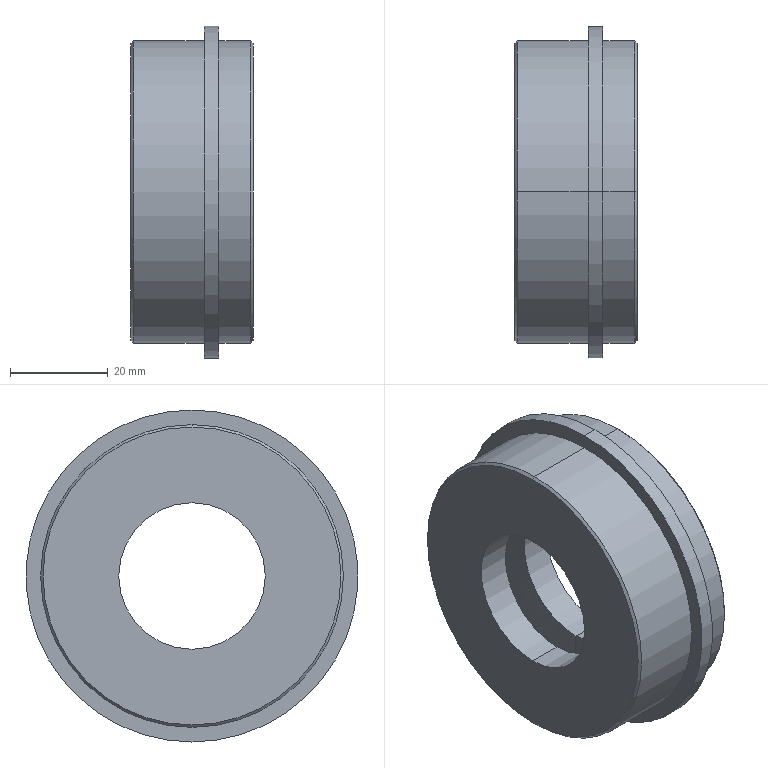Part | SolidWorks | features MBimport 1 | 1 solid | 29 faces | box 25 x 68 x 68 mm | volume 46745 mm3 | cylinder 14 | cone 8 | plane 5 | torus 2 | commonest cylinder face diameters 30 x4 62 x4 46 x2 52 x2 68 x2
STEP:
#1=CARTESIAN_POINT('',(25.,0.,-30.5));
#2=VERTEX_POINT('',#1);
#3=CARTESIAN_POINT('',(25.,0.,30.5));
#4=VERTEX_POINT('',#3);
#5=CARTESIAN_POINT('',(25.,0.,0.));
#6=DIRECTION('',(1.,0.,0.));
#7=DIRECTION('',(0.,0.,1.));
#8=AXIS2_PLACEMENT_3D('',#5,#6,#7);
#9=CIRCLE('',#8,30.5);
#10=EDGE_CURVE('',#2,#4,#9,.T.);
#11=ORIENTED_EDGE('',*,*,#10,.F.);
#12=CARTESIAN_POINT('',(24.5,0.,-31.));
#13=VERTEX_POINT('',#12);
#14=CARTESIAN_POINT('',(24.5,0.,-31.));
#15=DIRECTION('',(-0.7071,0.,-0.7071));
#16=VECTOR('',#15,1000.);
#17=LINE('',#14,#16);
#18=EDGE_CURVE('',#2,#13,#17,.T.);
#19=ORIENTED_EDGE('',*,*,#18,.T.);
#20=CARTESIAN_POINT('',(24.5,0.,31.));
#21=VERTEX_POINT('',#20);
#22=CARTESIAN_POINT('',(24.5,0.,0.));
#23=DIRECTION('',(-1.,0.,0.));
#24=DIRECTION('',(0.,0.,1.));
#25=AXIS2_PLACEMENT_3D('',#22,#23,#24);
#26=CIRCLE('',#25,31.);
#27=EDGE_CURVE('',#21,#13,#26,.T.);
#28=ORIENTED_EDGE('',*,*,#27,.F.);
#29=CARTESIAN_POINT('',(24.5,0.,31.));
#30=DIRECTION('',(-0.7071,0.,0.7071));
#31=VECTOR('',#30,1000.);
#32=LINE('',#29,#31);
#33=EDGE_CURVE('',#4,#21,#32,.T.);
#34=ORIENTED_EDGE('',*,*,#33,.F.);
#35=EDGE_LOOP('',(#11,#19,#28,#34));
#36=FACE_OUTER_BOUND('',#35,.T.);
#37=CARTESIAN_POINT('',(24.5,0.,0.));
#38=DIRECTION('',(-1.,0.,0.));
#39=DIRECTION('',(0.,0.,1.));
#40=AXIS2_PLACEMENT_3D('',#37,#38,#39);
#41=CONICAL_SURFACE('',#40,31.,0.7854);
#42=ADVANCED_FACE('',(#36),#41,.T.);
#43=CARTESIAN_POINT('',(0.,0.,30.5));
#44=VERTEX_POINT('',#43);
#45=CARTESIAN_POINT('',(0.,0.,-30.5));
#46=VERTEX_POINT('',#45);
#47=CARTESIAN_POINT('',(0.,0.,0.));
#48=DIRECTION('',(-1.,0.,0.));
#49=DIRECTION('',(0.,0.,-1.));
#50=AXIS2_PLACEMENT_3D('',#47,#48,#49);
#51=CIRCLE('',#50,30.5);
#52=EDGE_CURVE('',#44,#46,#51,.T.);
#53=ORIENTED_EDGE('',*,*,#52,.F.);
#54=CARTESIAN_POINT('',(0.5,0.,31.));
#55=VERTEX_POINT('',#54);
#56=CARTESIAN_POINT('',(0.,0.,30.5));
#57=DIRECTION('',(0.7071,0.,0.7071));
#58=VECTOR('',#57,1000.);
#59=LINE('',#56,#58);
#60=EDGE_CURVE('',#44,#55,#59,.T.);
#61=ORIENTED_EDGE('',*,*,#60,.T.);
#62=CARTESIAN_POINT('',(0.5,0.,-31.));
#63=VERTEX_POINT('',#62);
#64=CARTESIAN_POINT('',(0.5,0.,0.));
#65=DIRECTION('',(1.,0.,0.));
#66=DIRECTION('',(0.,0.,-1.));
#67=AXIS2_PLACEMENT_3D('',#64,#65,#66);
#68=CIRCLE('',#67,31.);
#69=EDGE_CURVE('',#63,#55,#68,.T.);
#70=ORIENTED_EDGE('',*,*,#69,.F.);
#71=CARTESIAN_POINT('',(0.,0.,-30.5));
#72=DIRECTION('',(0.7071,0.,-0.7071));
#73=VECTOR('',#72,1000.);
#74=LINE('',#71,#73);
#75=EDGE_CURVE('',#46,#63,#74,.T.);
#76=ORIENTED_EDGE('',*,*,#75,.F.);
#77=EDGE_LOOP('',(#53,#61,#70,#76));
#78=FACE_OUTER_BOUND('',#77,.T.);
#79=CARTESIAN_POINT('',(0.,0.,0.));
#80=DIRECTION('',(1.,0.,0.));
#81=DIRECTION('',(0.,0.,-1.));
#82=AXIS2_PLACEMENT_3D('',#79,#80,#81);
#83=CONICAL_SURFACE('',#82,30.5,0.7854);
#84=ADVANCED_FACE('',(#78),#83,.T.);
#85=CARTESIAN_POINT('',(21.,0.,-26.));
#86=VERTEX_POINT('',#85);
#87=CARTESIAN_POINT('',(21.,0.,26.));
#88=VERTEX_POINT('',#87);
#89=CARTESIAN_POINT('',(21.,0.,0.));
#90=DIRECTION('',(-1.,0.,0.));
#91=DIRECTION('',(0.,0.,1.));
#92=AXIS2_PLACEMENT_3D('',#89,#90,#91);
#93=CIRCLE('',#92,26.);
#94=EDGE_CURVE('',#86,#88,#93,.T.);
#95=ORIENTED_EDGE('',*,*,#94,.F.);
#96=CARTESIAN_POINT('',(19.,0.,-24.));
#97=VERTEX_POINT('',#96);
#98=CARTESIAN_POINT('',(21.,0.,-24.));
#99=DIRECTION('',(0.,1.,0.));
#100=DIRECTION('',(0.,0.,1.));
#101=AXIS2_PLACEMENT_3D('',#98,#99,#100);
#102=CIRCLE('',#101,2.);
#103=EDGE_CURVE('',#86,#97,#102,.T.);
#104=ORIENTED_EDGE('',*,*,#103,.T.);
#105=CARTESIAN_POINT('',(19.,0.,24.));
#106=VERTEX_POINT('',#105);
#107=CARTESIAN_POINT('',(19.,0.,0.));
#108=DIRECTION('',(1.,0.,0.));
#109=DIRECTION('',(0.,0.,1.));
#110=AXIS2_PLACEMENT_3D('',#107,#108,#109);
#111=CIRCLE('',#110,24.);
#112=EDGE_CURVE('',#106,#97,#111,.T.);
#113=ORIENTED_EDGE('',*,*,#112,.F.);
#114=CARTESIAN_POINT('',(21.,0.,24.));
#115=DIRECTION('',(0.,-1.,0.));
#116=DIRECTION('',(0.,0.,-1.));
#117=AXIS2_PLACEMENT_3D('',#114,#115,#116);
#118=CIRCLE('',#117,2.);
#119=EDGE_CURVE('',#88,#106,#118,.T.);
#120=ORIENTED_EDGE('',*,*,#119,.F.);
#121=EDGE_LOOP('',(#95,#104,#113,#120));
#122=FACE_OUTER_BOUND('',#121,.T.);
#123=CARTESIAN_POINT('',(21.,0.,0.));
#124=DIRECTION('',(-1.,0.,0.));
#125=DIRECTION('',(0.,0.,1.));
#126=AXIS2_PLACEMENT_3D('',#123,#124,#125);
#127=TOROIDAL_SURFACE('',#126,24.,2.);
#128=ADVANCED_FACE('',(#122),#127,.F.);
#129=CARTESIAN_POINT('',(15.,0.,31.));
#130=VERTEX_POINT('',#129);
#131=CARTESIAN_POINT('',(15.,0.,-31.));
#132=VERTEX_POINT('',#131);
#133=CARTESIAN_POINT('',(15.,0.,0.));
#134=DIRECTION('',(-1.,0.,0.));
#135=DIRECTION('',(0.,0.,1.));
#136=AXIS2_PLACEMENT_3D('',#133,#134,#135);
#137=CIRCLE('',#136,31.);
#138=EDGE_CURVE('',#130,#132,#137,.T.);
#139=ORIENTED_EDGE('',*,*,#138,.T.);
#140=CARTESIAN_POINT('',(0.,0.,-31.));
#141=DIRECTION('',(-1.,0.,0.));
#142=VECTOR('',#141,1000.);
#143=LINE('',#140,#142);
#144=EDGE_CURVE('',#132,#63,#143,.T.);
#145=ORIENTED_EDGE('',*,*,#144,.T.);
#146=ORIENTED_EDGE('',*,*,#69,.T.);
#147=CARTESIAN_POINT('',(0.,0.,31.));
#148=DIRECTION('',(-1.,0.,0.));
#149=VECTOR('',#148,1000.);
#150=LINE('',#147,#149);
#151=EDGE_CURVE('',#130,#55,#150,.T.);
#152=ORIENTED_EDGE('',*,*,#151,.F.);
#153=EDGE_LOOP('',(#139,#145,#146,#152));
#154=FACE_OUTER_BOUND('',#153,.T.);
#155=CARTESIAN_POINT('',(0.,0.,0.));
#156=DIRECTION('',(-1.,0.,0.));
#157=DIRECTION('',(0.,0.,1.));
#158=AXIS2_PLACEMENT_3D('',#155,#156,#157);
#159=CYLINDRICAL_SURFACE('',#158,31.);
#160=ADVANCED_FACE('',(#154),#159,.T.);
#161=CARTESIAN_POINT('',(18.,0.,34.));
#162=VERTEX_POINT('',#161);
#163=CARTESIAN_POINT('',(18.,0.,-34.));
#164=VERTEX_POINT('',#163);
#165=CARTESIAN_POINT('',(18.,0.,0.));
#166=DIRECTION('',(-1.,0.,0.));
#167=DIRECTION('',(0.,0.,1.));
#168=AXIS2_PLACEMENT_3D('',#165,#166,#167);
#169=CIRCLE('',#168,34.);
#170=EDGE_CURVE('',#162,#164,#169,.T.);
#171=ORIENTED_EDGE('',*,*,#170,.T.);
#172=CARTESIAN_POINT('',(15.,0.,-34.));
#173=VERTEX_POINT('',#172);
#174=CARTESIAN_POINT('',(0.,0.,-34.));
#175=DIRECTION('',(-1.,0.,0.));
#176=VECTOR('',#175,1000.);
#177=LINE('',#174,#176);
#178=EDGE_CURVE('',#164,#173,#177,.T.);
#179=ORIENTED_EDGE('',*,*,#178,.T.);
#180=CARTESIAN_POINT('',(15.,0.,34.));
#181=VERTEX_POINT('',#180);
#182=CARTESIAN_POINT('',(15.,0.,0.));
#183=DIRECTION('',(-1.,0.,0.));
#184=DIRECTION('',(0.,0.,1.));
#185=AXIS2_PLACEMENT_3D('',#182,#183,#184);
#186=CIRCLE('',#185,34.);
#187=EDGE_CURVE('',#181,#173,#186,.T.);
#188=ORIENTED_EDGE('',*,*,#187,.F.);
#189=CARTESIAN_POINT('',(0.,0.,34.));
#190=DIRECTION('',(-1.,0.,0.));
#191=VECTOR('',#190,1000.);
#192=LINE('',#189,#191);
#193=EDGE_CURVE('',#162,#181,#192,.T.);
#194=ORIENTED_EDGE('',*,*,#193,.F.);
#195=EDGE_LOOP('',(#171,#179,#188,#194));
#196=FACE_OUTER_BOUND('',#195,.T.);
#197=CARTESIAN_POINT('',(0.,0.,0.));
#198=DIRECTION('',(-1.,0.,0.));
#199=DIRECTION('',(0.,0.,1.));
#200=AXIS2_PLACEMENT_3D('',#197,#198,#199);
#201=CYLINDRICAL_SURFACE('',#200,34.);
#202=ADVANCED_FACE('',(#196),#201,.T.);
#203=ORIENTED_EDGE('',*,*,#27,.T.);
#204=CARTESIAN_POINT('',(18.,0.,-31.));
#205=VERTEX_POINT('',#204);
#206=CARTESIAN_POINT('',(0.,0.,-31.));
#207=DIRECTION('',(-1.,0.,0.));
#208=VECTOR('',#207,1000.);
#209=LINE('',#206,#208);
#210=EDGE_CURVE('',#13,#205,#209,.T.);
#211=ORIENTED_EDGE('',*,*,#210,.T.);
#212=CARTESIAN_POINT('',(18.,0.,31.));
#213=VERTEX_POINT('',#212);
#214=CARTESIAN_POINT('',(18.,0.,0.));
#215=DIRECTION('',(-1.,0.,0.));
#216=DIRECTION('',(0.,0.,1.));
#217=AXIS2_PLACEMENT_3D('',#214,#215,#216);
#218=CIRCLE('',#217,31.);
#219=EDGE_CURVE('',#213,#205,#218,.T.);
#220=ORIENTED_EDGE('',*,*,#219,.F.);
#221=CARTESIAN_POINT('',(0.,0.,31.));
#222=DIRECTION('',(-1.,0.,0.));
#223=VECTOR('',#222,1000.);
#224=LINE('',#221,#223);
#225=EDGE_CURVE('',#21,#213,#224,.T.);
#226=ORIENTED_EDGE('',*,*,#225,.F.);
#227=EDGE_LOOP('',(#203,#211,#220,#226));
#228=FACE_OUTER_BOUND('',#227,.T.);
#229=CARTESIAN_POINT('',(0.,0.,0.));
#230=DIRECTION('',(-1.,0.,0.));
#231=DIRECTION('',(0.,0.,1.));
#232=AXIS2_PLACEMENT_3D('',#229,#230,#231);
#233=CYLINDRICAL_SURFACE('',#232,31.);
#234=ADVANCED_FACE('',(#228),#233,.T.);
#235=CARTESIAN_POINT('',(25.,0.,-26.));
#236=VERTEX_POINT('',#235);
#237=CARTESIAN_POINT('',(25.,0.,26.));
#238=VERTEX_POINT('',#237);
#239=CARTESIAN_POINT('',(25.,0.,0.));
#240=DIRECTION('',(-1.,0.,0.));
#241=DIRECTION('',(0.,0.,1.));
#242=AXIS2_PLACEMENT_3D('',#239,#240,#241);
#243=CIRCLE('',#242,26.);
#244=EDGE_CURVE('',#236,#238,#243,.T.);
#245=ORIENTED_EDGE('',*,*,#244,.F.);
#246=CARTESIAN_POINT('',(0.,0.,-26.));
#247=DIRECTION('',(-1.,0.,0.));
#248=VECTOR('',#247,1000.);
#249=LINE('',#246,#248);
#250=EDGE_CURVE('',#236,#86,#249,.T.);
#251=ORIENTED_EDGE('',*,*,#250,.T.);
#252=ORIENTED_EDGE('',*,*,#94,.T.);
#253=CARTESIAN_POINT('',(0.,0.,26.));
#254=DIRECTION('',(-1.,0.,0.));
#255=VECTOR('',#254,1000.);
#256=LINE('',#253,#255);
#257=EDGE_CURVE('',#238,#88,#256,.T.);
#258=ORIENTED_EDGE('',*,*,#257,.F.);
#259=EDGE_LOOP('',(#245,#251,#252,#258));
#260=FACE_OUTER_BOUND('',#259,.T.);
#261=CARTESIAN_POINT('',(0.,0.,0.));
#262=DIRECTION('',(-1.,0.,0.));
#263=DIRECTION('',(0.,0.,1.));
#264=AXIS2_PLACEMENT_3D('',#261,#262,#263);
#265=CYLINDRICAL_SURFACE('',#264,26.);
#266=ADVANCED_FACE('',(#260),#265,.F.);
#267=CARTESIAN_POINT('',(19.,0.,-15.));
#268=VERTEX_POINT('',#267);
#269=CARTESIAN_POINT('',(19.,0.,15.));
#270=VERTEX_POINT('',#269);
#271=CARTESIAN_POINT('',(19.,0.,0.));
#272=DIRECTION('',(-1.,0.,0.));
#273=DIRECTION('',(0.,0.,1.));
#274=AXIS2_PLACEMENT_3D('',#271,#272,#273);
#275=CIRCLE('',#274,15.);
#276=EDGE_CURVE('',#268,#270,#275,.T.);
#277=ORIENTED_EDGE('',*,*,#276,.F.);
#278=CARTESIAN_POINT('',(12.5,0.,-15.));
#279=VERTEX_POINT('',#278);
#280=CARTESIAN_POINT('',(0.,0.,-15.));
#281=DIRECTION('',(-1.,0.,0.));
#282=VECTOR('',#281,1000.);
#283=LINE('',#280,#282);
#284=EDGE_CURVE('',#268,#279,#283,.T.);
#285=ORIENTED_EDGE('',*,*,#284,.T.);
#286=CARTESIAN_POINT('',(12.5,0.,15.));
#287=VERTEX_POINT('',#286);
#288=CARTESIAN_POINT('',(12.5,0.,0.));
#289=DIRECTION('',(-1.,0.,0.));
#290=DIRECTION('',(0.,0.,1.));
#291=AXIS2_PLACEMENT_3D('',#288,#289,#290);
#292=CIRCLE('',#291,15.);
#293=EDGE_CURVE('',#279,#287,#292,.T.);
#294=ORIENTED_EDGE('',*,*,#293,.T.);
#295=CARTESIAN_POINT('',(0.,0.,15.));
#296=DIRECTION('',(-1.,0.,0.));
#297=VECTOR('',#296,1000.);
#298=LINE('',#295,#297);
#299=EDGE_CURVE('',#270,#287,#298,.T.);
#300=ORIENTED_EDGE('',*,*,#299,.F.);
#301=EDGE_LOOP('',(#277,#285,#294,#300));
#302=FACE_OUTER_BOUND('',#301,.T.);
#303=CARTESIAN_POINT('',(0.,0.,0.));
#304=DIRECTION('',(-1.,0.,0.));
#305=DIRECTION('',(0.,0.,1.));
#306=AXIS2_PLACEMENT_3D('',#303,#304,#305);
#307=CYLINDRICAL_SURFACE('',#306,15.);
#308=ADVANCED_FACE('',(#302),#307,.F.);
#309=ORIENTED_EDGE('',*,*,#293,.F.);
#310=CARTESIAN_POINT('',(11.75,0.,-23.));
#311=VERTEX_POINT('',#310);
#312=CARTESIAN_POINT('',(11.75,0.,-23.));
#313=DIRECTION('',(-0.09334,0.,-0.9956));
#314=VECTOR('',#313,1000.);
#315=LINE('',#312,#314);
#316=EDGE_CURVE('',#279,#311,#315,.T.);
#317=ORIENTED_EDGE('',*,*,#316,.T.);
#318=CARTESIAN_POINT('',(11.75,0.,23.));
#319=VERTEX_POINT('',#318);
#320=CARTESIAN_POINT('',(11.75,0.,0.));
#321=DIRECTION('',(-1.,0.,0.));
#322=DIRECTION('',(0.,0.,1.));
#323=AXIS2_PLACEMENT_3D('',#320,#321,#322);
#324=CIRCLE('',#323,23.);
#325=EDGE_CURVE('',#311,#319,#324,.T.);
#326=ORIENTED_EDGE('',*,*,#325,.T.);
#327=CARTESIAN_POINT('',(11.75,0.,23.));
#328=DIRECTION('',(-0.09334,0.,0.9956));
#329=VECTOR('',#328,1000.);
#330=LINE('',#327,#329);
#331=EDGE_CURVE('',#287,#319,#330,.T.);
#332=ORIENTED_EDGE('',*,*,#331,.F.);
#333=EDGE_LOOP('',(#309,#317,#326,#332));
#334=FACE_OUTER_BOUND('',#333,.T.);
#335=CARTESIAN_POINT('',(11.75,0.,0.));
#336=DIRECTION('',(-1.,0.,0.));
#337=DIRECTION('',(0.,0.,1.));
#338=AXIS2_PLACEMENT_3D('',#335,#336,#337);
#339=CONICAL_SURFACE('',#338,23.,1.477);
#340=ADVANCED_FACE('',(#334),#339,.F.);
#341=ORIENTED_EDGE('',*,*,#325,.F.);
#342=CARTESIAN_POINT('',(7.75,0.,-23.));
#343=VERTEX_POINT('',#342);
#344=CARTESIAN_POINT('',(0.,0.,-23.));
#345=DIRECTION('',(-1.,0.,0.));
#346=VECTOR('',#345,1000.);
#347=LINE('',#344,#346);
#348=EDGE_CURVE('',#311,#343,#347,.T.);
#349=ORIENTED_EDGE('',*,*,#348,.T.);
#350=CARTESIAN_POINT('',(7.75,0.,23.));
#351=VERTEX_POINT('',#350);
#352=CARTESIAN_POINT('',(7.75,0.,0.));
#353=DIRECTION('',(-1.,0.,0.));
#354=DIRECTION('',(0.,0.,1.));
#355=AXIS2_PLACEMENT_3D('',#352,#353,#354);
#356=CIRCLE('',#355,23.);
#357=EDGE_CURVE('',#343,#351,#356,.T.);
#358=ORIENTED_EDGE('',*,*,#357,.T.);
#359=CARTESIAN_POINT('',(0.,0.,23.));
#360=DIRECTION('',(-1.,0.,0.));
#361=VECTOR('',#360,1000.);
#362=LINE('',#359,#361);
#363=EDGE_CURVE('',#319,#351,#362,.T.);
#364=ORIENTED_EDGE('',*,*,#363,.F.);
#365=EDGE_LOOP('',(#341,#349,#358,#364));
#366=FACE_OUTER_BOUND('',#365,.T.);
#367=CARTESIAN_POINT('',(0.,0.,0.));
#368=DIRECTION('',(-1.,0.,0.));
#369=DIRECTION('',(0.,0.,1.));
#370=AXIS2_PLACEMENT_3D('',#367,#368,#369);
#371=CYLINDRICAL_SURFACE('',#370,23.);
#372=ADVANCED_FACE('',(#366),#371,.F.);
#373=CARTESIAN_POINT('',(7.,0.,-15.));
#374=VERTEX_POINT('',#373);
#375=CARTESIAN_POINT('',(7.,0.,15.));
#376=VERTEX_POINT('',#375);
#377=CARTESIAN_POINT('',(7.,0.,0.));
#378=DIRECTION('',(-1.,0.,0.));
#379=DIRECTION('',(0.,0.,1.));
#380=AXIS2_PLACEMENT_3D('',#377,#378,#379);
#381=CIRCLE('',#380,15.);
#382=EDGE_CURVE('',#374,#376,#381,.T.);
#383=ORIENTED_EDGE('',*,*,#382,.T.);
#384=CARTESIAN_POINT('',(7.,0.,15.));
#385=DIRECTION('',(0.09334,0.,0.9956));
#386=VECTOR('',#385,1000.);
#387=LINE('',#384,#386);
#388=EDGE_CURVE('',#376,#351,#387,.T.);
#389=ORIENTED_EDGE('',*,*,#388,.T.);
#390=ORIENTED_EDGE('',*,*,#357,.F.);
#391=CARTESIAN_POINT('',(7.,0.,-15.));
#392=DIRECTION('',(0.09334,0.,-0.9956));
#393=VECTOR('',#392,1000.);
#394=LINE('',#391,#393);
#395=EDGE_CURVE('',#374,#343,#394,.T.);
#396=ORIENTED_EDGE('',*,*,#395,.F.);
#397=EDGE_LOOP('',(#383,#389,#390,#396));
#398=FACE_OUTER_BOUND('',#397,.T.);
#399=CARTESIAN_POINT('',(7.,0.,0.));
#400=DIRECTION('',(1.,0.,0.));
#401=DIRECTION('',(0.,0.,-1.));
#402=AXIS2_PLACEMENT_3D('',#399,#400,#401);
#403=CONICAL_SURFACE('',#402,15.,1.477);
#404=ADVANCED_FACE('',(#398),#403,.F.);
#405=ORIENTED_EDGE('',*,*,#382,.F.);
#406=CARTESIAN_POINT('',(0.,0.,-15.));
#407=VERTEX_POINT('',#406);
#408=CARTESIAN_POINT('',(0.,0.,-15.));
#409=DIRECTION('',(-1.,0.,0.));
#410=VECTOR('',#409,1000.);
#411=LINE('',#408,#410);
#412=EDGE_CURVE('',#374,#407,#411,.T.);
#413=ORIENTED_EDGE('',*,*,#412,.T.);
#414=CARTESIAN_POINT('',(0.,0.,15.));
#415=VERTEX_POINT('',#414);
#416=CARTESIAN_POINT('',(0.,0.,0.));
#417=DIRECTION('',(-1.,0.,0.));
#418=DIRECTION('',(0.,0.,1.));
#419=AXIS2_PLACEMENT_3D('',#416,#417,#418);
#420=CIRCLE('',#419,15.);
#421=EDGE_CURVE('',#407,#415,#420,.T.);
#422=ORIENTED_EDGE('',*,*,#421,.T.);
#423=CARTESIAN_POINT('',(0.,0.,15.));
#424=DIRECTION('',(-1.,0.,0.));
#425=VECTOR('',#424,1000.);
#426=LINE('',#423,#425);
#427=EDGE_CURVE('',#376,#415,#426,.T.);
#428=ORIENTED_EDGE('',*,*,#427,.F.);
#429=EDGE_LOOP('',(#405,#413,#422,#428));
#430=FACE_OUTER_BOUND('',#429,.T.);
#431=CARTESIAN_POINT('',(0.,0.,0.));
#432=DIRECTION('',(-1.,0.,0.));
#433=DIRECTION('',(0.,0.,1.));
#434=AXIS2_PLACEMENT_3D('',#431,#432,#433);
#435=CYLINDRICAL_SURFACE('',#434,15.);
#436=ADVANCED_FACE('',(#430),#435,.F.);
#437=CARTESIAN_POINT('',(0.,0.,0.));
#438=DIRECTION('',(-1.,0.,0.));
#439=DIRECTION('',(0.,0.,-1.));
#440=AXIS2_PLACEMENT_3D('',#437,#438,#439);
#441=CIRCLE('',#440,30.5);
#442=EDGE_CURVE('',#46,#44,#441,.T.);
#443=ORIENTED_EDGE('',*,*,#442,.T.);
#444=ORIENTED_EDGE('',*,*,#52,.T.);
#445=EDGE_LOOP('',(#443,#444));
#446=FACE_OUTER_BOUND('',#445,.T.);
#447=CARTESIAN_POINT('',(0.,0.,0.));
#448=DIRECTION('',(-1.,0.,0.));
#449=DIRECTION('',(0.,0.,1.));
#450=AXIS2_PLACEMENT_3D('',#447,#448,#449);
#451=CIRCLE('',#450,15.);
#452=EDGE_CURVE('',#415,#407,#451,.T.);
#453=ORIENTED_EDGE('',*,*,#452,.F.);
#454=ORIENTED_EDGE('',*,*,#421,.F.);
#455=EDGE_LOOP('',(#453,#454));
#456=FACE_BOUND('',#455,.T.);
#457=CARTESIAN_POINT('',(0.,31.,0.));
#458=DIRECTION('',(1.,0.,0.));
#459=DIRECTION('',(0.,1.,0.));
#460=AXIS2_PLACEMENT_3D('',#457,#458,#459);
#461=PLANE('',#460);
#462=ADVANCED_FACE('',(#446,#456),#461,.F.);
#463=ORIENTED_EDGE('',*,*,#412,.F.);
#464=CARTESIAN_POINT('',(7.,0.,0.));
#465=DIRECTION('',(-1.,0.,0.));
#466=DIRECTION('',(0.,0.,1.));
#467=AXIS2_PLACEMENT_3D('',#464,#465,#466);
#468=CIRCLE('',#467,15.);
#469=EDGE_CURVE('',#376,#374,#468,.T.);
#470=ORIENTED_EDGE('',*,*,#469,.F.);
#471=ORIENTED_EDGE('',*,*,#427,.T.);
#472=ORIENTED_EDGE('',*,*,#452,.T.);
#473=EDGE_LOOP('',(#463,#470,#471,#472));
#474=FACE_OUTER_BOUND('',#473,.T.);
#475=CARTESIAN_POINT('',(0.,0.,0.));
#476=DIRECTION('',(-1.,0.,0.));
#477=DIRECTION('',(0.,0.,1.));
#478=AXIS2_PLACEMENT_3D('',#475,#476,#477);
#479=CYLINDRICAL_SURFACE('',#478,15.);
#480=ADVANCED_FACE('',(#474),#479,.F.);
#481=ORIENTED_EDGE('',*,*,#388,.F.);
#482=ORIENTED_EDGE('',*,*,#469,.T.);
#483=ORIENTED_EDGE('',*,*,#395,.T.);
#484=CARTESIAN_POINT('',(7.75,0.,0.));
#485=DIRECTION('',(-1.,0.,0.));
#486=DIRECTION('',(0.,0.,1.));
#487=AXIS2_PLACEMENT_3D('',#484,#485,#486);
#488=CIRCLE('',#487,23.);
#489=EDGE_CURVE('',#351,#343,#488,.T.);
#490=ORIENTED_EDGE('',*,*,#489,.F.);
#491=EDGE_LOOP('',(#481,#482,#483,#490));
#492=FACE_OUTER_BOUND('',#491,.T.);
#493=CARTESIAN_POINT('',(7.,0.,0.));
#494=DIRECTION('',(1.,0.,0.));
#495=DIRECTION('',(0.,0.,-1.));
#496=AXIS2_PLACEMENT_3D('',#493,#494,#495);
#497=CONICAL_SURFACE('',#496,15.,1.477);
#498=ADVANCED_FACE('',(#492),#497,.F.);
#499=ORIENTED_EDGE('',*,*,#348,.F.);
#500=CARTESIAN_POINT('',(11.75,0.,0.));
#501=DIRECTION('',(-1.,0.,0.));
#502=DIRECTION('',(0.,0.,1.));
#503=AXIS2_PLACEMENT_3D('',#500,#501,#502);
#504=CIRCLE('',#503,23.);
#505=EDGE_CURVE('',#319,#311,#504,.T.);
#506=ORIENTED_EDGE('',*,*,#505,.F.);
#507=ORIENTED_EDGE('',*,*,#363,.T.);
#508=ORIENTED_EDGE('',*,*,#489,.T.);
#509=EDGE_LOOP('',(#499,#506,#507,#508));
#510=FACE_OUTER_BOUND('',#509,.T.);
#511=CARTESIAN_POINT('',(0.,0.,0.));
#512=DIRECTION('',(-1.,0.,0.));
#513=DIRECTION('',(0.,0.,1.));
#514=AXIS2_PLACEMENT_3D('',#511,#512,#513);
#515=CYLINDRICAL_SURFACE('',#514,23.);
#516=ADVANCED_FACE('',(#510),#515,.F.);
#517=ORIENTED_EDGE('',*,*,#316,.F.);
#518=CARTESIAN_POINT('',(12.5,0.,0.));
#519=DIRECTION('',(-1.,0.,0.));
#520=DIRECTION('',(0.,0.,1.));
#521=AXIS2_PLACEMENT_3D('',#518,#519,#520);
#522=CIRCLE('',#521,15.);
#523=EDGE_CURVE('',#287,#279,#522,.T.);
#524=ORIENTED_EDGE('',*,*,#523,.F.);
#525=ORIENTED_EDGE('',*,*,#331,.T.);
#526=ORIENTED_EDGE('',*,*,#505,.T.);
#527=EDGE_LOOP('',(#517,#524,#525,#526));
#528=FACE_OUTER_BOUND('',#527,.T.);
#529=CARTESIAN_POINT('',(11.75,0.,0.));
#530=DIRECTION('',(-1.,0.,0.));
#531=DIRECTION('',(0.,0.,1.));
#532=AXIS2_PLACEMENT_3D('',#529,#530,#531);
#533=CONICAL_SURFACE('',#532,23.,1.477);
#534=ADVANCED_FACE('',(#528),#533,.F.);
#535=ORIENTED_EDGE('',*,*,#284,.F.);
#536=CARTESIAN_POINT('',(19.,0.,0.));
#537=DIRECTION('',(-1.,0.,0.));
#538=DIRECTION('',(0.,0.,1.));
#539=AXIS2_PLACEMENT_3D('',#536,#537,#538);
#540=CIRCLE('',#539,15.);
#541=EDGE_CURVE('',#270,#268,#540,.T.);
#542=ORIENTED_EDGE('',*,*,#541,.F.);
#543=ORIENTED_EDGE('',*,*,#299,.T.);
#544=ORIENTED_EDGE('',*,*,#523,.T.);
#545=EDGE_LOOP('',(#535,#542,#543,#544));
#546=FACE_OUTER_BOUND('',#545,.T.);
#547=CARTESIAN_POINT('',(0.,0.,0.));
#548=DIRECTION('',(-1.,0.,0.));
#549=DIRECTION('',(0.,0.,1.));
#550=AXIS2_PLACEMENT_3D('',#547,#548,#549);
#551=CYLINDRICAL_SURFACE('',#550,15.);
#552=ADVANCED_FACE('',(#546),#551,.F.);
#553=ORIENTED_EDGE('',*,*,#112,.T.);
#554=CARTESIAN_POINT('',(19.,0.,0.));
#555=DIRECTION('',(1.,0.,0.));
#556=DIRECTION('',(0.,0.,1.));
#557=AXIS2_PLACEMENT_3D('',#554,#555,#556);
#558=CIRCLE('',#557,24.);
#559=EDGE_CURVE('',#97,#106,#558,.T.);
#560=ORIENTED_EDGE('',*,*,#559,.T.);
#561=EDGE_LOOP('',(#553,#560));
#562=FACE_OUTER_BOUND('',#561,.T.);
#563=ORIENTED_EDGE('',*,*,#541,.T.);
#564=ORIENTED_EDGE('',*,*,#276,.T.);
#565=EDGE_LOOP('',(#563,#564));
#566=FACE_BOUND('',#565,.T.);
#567=CARTESIAN_POINT('',(19.,15.,0.));
#568=DIRECTION('',(-1.,0.,0.));
#569=DIRECTION('',(0.,0.,1.));
#570=AXIS2_PLACEMENT_3D('',#567,#568,#569);
#571=PLANE('',#570);
#572=ADVANCED_FACE('',(#562,#566),#571,.F.);
#573=ORIENTED_EDGE('',*,*,#250,.F.);
#574=CARTESIAN_POINT('',(25.,0.,0.));
#575=DIRECTION('',(-1.,0.,0.));
#576=DIRECTION('',(0.,0.,1.));
#577=AXIS2_PLACEMENT_3D('',#574,#575,#576);
#578=CIRCLE('',#577,26.);
#579=EDGE_CURVE('',#238,#236,#578,.T.);
#580=ORIENTED_EDGE('',*,*,#579,.F.);
#581=ORIENTED_EDGE('',*,*,#257,.T.);
#582=CARTESIAN_POINT('',(21.,0.,0.));
#583=DIRECTION('',(-1.,0.,0.));
#584=DIRECTION('',(0.,0.,1.));
#585=AXIS2_PLACEMENT_3D('',#582,#583,#584);
#586=CIRCLE('',#585,26.);
#587=EDGE_CURVE('',#88,#86,#586,.T.);
#588=ORIENTED_EDGE('',*,*,#587,.T.);
#589=EDGE_LOOP('',(#573,#580,#581,#588));
#590=FACE_OUTER_BOUND('',#589,.T.);
#591=CARTESIAN_POINT('',(0.,0.,0.));
#592=DIRECTION('',(-1.,0.,0.));
#593=DIRECTION('',(0.,0.,1.));
#594=AXIS2_PLACEMENT_3D('',#591,#592,#593);
#595=CYLINDRICAL_SURFACE('',#594,26.);
#596=ADVANCED_FACE('',(#590),#595,.F.);
#597=CARTESIAN_POINT('',(25.,0.,0.));
#598=DIRECTION('',(1.,0.,0.));
#599=DIRECTION('',(0.,0.,1.));
#600=AXIS2_PLACEMENT_3D('',#597,#598,#599);
#601=CIRCLE('',#600,30.5);
#602=EDGE_CURVE('',#4,#2,#601,.T.);
#603=ORIENTED_EDGE('',*,*,#602,.T.);
#604=ORIENTED_EDGE('',*,*,#10,.T.);
#605=EDGE_LOOP('',(#603,#604));
#606=FACE_OUTER_BOUND('',#605,.T.);
#607=ORIENTED_EDGE('',*,*,#579,.T.);
#608=ORIENTED_EDGE('',*,*,#244,.T.);
#609=EDGE_LOOP('',(#607,#608));
#610=FACE_BOUND('',#609,.T.);
#611=CARTESIAN_POINT('',(25.,26.,0.));
#612=DIRECTION('',(-1.,0.,0.));
#613=DIRECTION('',(0.,0.,1.));
#614=AXIS2_PLACEMENT_3D('',#611,#612,#613);
#615=PLANE('',#614);
#616=ADVANCED_FACE('',(#606,#610),#615,.F.);
#617=ORIENTED_EDGE('',*,*,#210,.F.);
#618=CARTESIAN_POINT('',(24.5,0.,0.));
#619=DIRECTION('',(-1.,0.,0.));
#620=DIRECTION('',(0.,0.,1.));
#621=AXIS2_PLACEMENT_3D('',#618,#619,#620);
#622=CIRCLE('',#621,31.);
#623=EDGE_CURVE('',#13,#21,#622,.T.);
#624=ORIENTED_EDGE('',*,*,#623,.T.);
#625=ORIENTED_EDGE('',*,*,#225,.T.);
#626=CARTESIAN_POINT('',(18.,0.,0.));
#627=DIRECTION('',(-1.,0.,0.));
#628=DIRECTION('',(0.,0.,1.));
#629=AXIS2_PLACEMENT_3D('',#626,#627,#628);
#630=CIRCLE('',#629,31.);
#631=EDGE_CURVE('',#205,#213,#630,.T.);
#632=ORIENTED_EDGE('',*,*,#631,.F.);
#633=EDGE_LOOP('',(#617,#624,#625,#632));
#634=FACE_OUTER_BOUND('',#633,.T.);
#635=CARTESIAN_POINT('',(0.,0.,0.));
#636=DIRECTION('',(-1.,0.,0.));
#637=DIRECTION('',(0.,0.,1.));
#638=AXIS2_PLACEMENT_3D('',#635,#636,#637);
#639=CYLINDRICAL_SURFACE('',#638,31.);
#640=ADVANCED_FACE('',(#634),#639,.T.);
#641=ORIENTED_EDGE('',*,*,#170,.F.);
#642=CARTESIAN_POINT('',(18.,0.,0.));
#643=DIRECTION('',(-1.,0.,0.));
#644=DIRECTION('',(0.,0.,1.));
#645=AXIS2_PLACEMENT_3D('',#642,#643,#644);
#646=CIRCLE('',#645,34.);
#647=EDGE_CURVE('',#164,#162,#646,.T.);
#648=ORIENTED_EDGE('',*,*,#647,.F.);
#649=EDGE_LOOP('',(#641,#648));
#650=FACE_OUTER_BOUND('',#649,.T.);
#651=ORIENTED_EDGE('',*,*,#219,.T.);
#652=ORIENTED_EDGE('',*,*,#631,.T.);
#653=EDGE_LOOP('',(#651,#652));
#654=FACE_BOUND('',#653,.T.);
#655=CARTESIAN_POINT('',(18.,31.,0.));
#656=DIRECTION('',(-1.,0.,0.));
#657=DIRECTION('',(0.,0.,1.));
#658=AXIS2_PLACEMENT_3D('',#655,#656,#657);
#659=PLANE('',#658);
#660=ADVANCED_FACE('',(#650,#654),#659,.F.);
#661=ORIENTED_EDGE('',*,*,#178,.F.);
#662=ORIENTED_EDGE('',*,*,#647,.T.);
#663=ORIENTED_EDGE('',*,*,#193,.T.);
#664=CARTESIAN_POINT('',(15.,0.,0.));
#665=DIRECTION('',(-1.,0.,0.));
#666=DIRECTION('',(0.,0.,1.));
#667=AXIS2_PLACEMENT_3D('',#664,#665,#666);
#668=CIRCLE('',#667,34.);
#669=EDGE_CURVE('',#173,#181,#668,.T.);
#670=ORIENTED_EDGE('',*,*,#669,.F.);
#671=EDGE_LOOP('',(#661,#662,#663,#670));
#672=FACE_OUTER_BOUND('',#671,.T.);
#673=CARTESIAN_POINT('',(0.,0.,0.));
#674=DIRECTION('',(-1.,0.,0.));
#675=DIRECTION('',(0.,0.,1.));
#676=AXIS2_PLACEMENT_3D('',#673,#674,#675);
#677=CYLINDRICAL_SURFACE('',#676,34.);
#678=ADVANCED_FACE('',(#672),#677,.T.);
#679=ORIENTED_EDGE('',*,*,#138,.F.);
#680=CARTESIAN_POINT('',(15.,0.,0.));
#681=DIRECTION('',(-1.,0.,0.));
#682=DIRECTION('',(0.,0.,1.));
#683=AXIS2_PLACEMENT_3D('',#680,#681,#682);
#684=CIRCLE('',#683,31.);
#685=EDGE_CURVE('',#132,#130,#684,.T.);
#686=ORIENTED_EDGE('',*,*,#685,.F.);
#687=EDGE_LOOP('',(#679,#686));
#688=FACE_BOUND('',#687,.T.);
#689=ORIENTED_EDGE('',*,*,#187,.T.);
#690=ORIENTED_EDGE('',*,*,#669,.T.);
#691=EDGE_LOOP('',(#689,#690));
#692=FACE_OUTER_BOUND('',#691,.T.);
#693=CARTESIAN_POINT('',(15.,34.,0.));
#694=DIRECTION('',(1.,0.,0.));
#695=DIRECTION('',(0.,1.,0.));
#696=AXIS2_PLACEMENT_3D('',#693,#694,#695);
#697=PLANE('',#696);
#698=ADVANCED_FACE('',(#688,#692),#697,.F.);
#699=ORIENTED_EDGE('',*,*,#144,.F.);
#700=ORIENTED_EDGE('',*,*,#685,.T.);
#701=ORIENTED_EDGE('',*,*,#151,.T.);
#702=CARTESIAN_POINT('',(0.5,0.,0.));
#703=DIRECTION('',(1.,0.,0.));
#704=DIRECTION('',(0.,0.,-1.));
#705=AXIS2_PLACEMENT_3D('',#702,#703,#704);
#706=CIRCLE('',#705,31.);
#707=EDGE_CURVE('',#55,#63,#706,.T.);
#708=ORIENTED_EDGE('',*,*,#707,.T.);
#709=EDGE_LOOP('',(#699,#700,#701,#708));
#710=FACE_OUTER_BOUND('',#709,.T.);
#711=CARTESIAN_POINT('',(0.,0.,0.));
#712=DIRECTION('',(-1.,0.,0.));
#713=DIRECTION('',(0.,0.,1.));
#714=AXIS2_PLACEMENT_3D('',#711,#712,#713);
#715=CYLINDRICAL_SURFACE('',#714,31.);
#716=ADVANCED_FACE('',(#710),#715,.T.);
#717=ORIENTED_EDGE('',*,*,#103,.F.);
#718=ORIENTED_EDGE('',*,*,#587,.F.);
#719=ORIENTED_EDGE('',*,*,#119,.T.);
#720=ORIENTED_EDGE('',*,*,#559,.F.);
#721=EDGE_LOOP('',(#717,#718,#719,#720));
#722=FACE_OUTER_BOUND('',#721,.T.);
#723=CARTESIAN_POINT('',(21.,0.,0.));
#724=DIRECTION('',(-1.,0.,0.));
#725=DIRECTION('',(0.,0.,1.));
#726=AXIS2_PLACEMENT_3D('',#723,#724,#725);
#727=TOROIDAL_SURFACE('',#726,24.,2.);
#728=ADVANCED_FACE('',(#722),#727,.F.);
#729=ORIENTED_EDGE('',*,*,#60,.F.);
#730=ORIENTED_EDGE('',*,*,#442,.F.);
#731=ORIENTED_EDGE('',*,*,#75,.T.);
#732=ORIENTED_EDGE('',*,*,#707,.F.);
#733=EDGE_LOOP('',(#729,#730,#731,#732));
#734=FACE_OUTER_BOUND('',#733,.T.);
#735=CARTESIAN_POINT('',(0.,0.,0.));
#736=DIRECTION('',(1.,0.,0.));
#737=DIRECTION('',(0.,0.,-1.));
#738=AXIS2_PLACEMENT_3D('',#735,#736,#737);
#739=CONICAL_SURFACE('',#738,30.5,0.7854);
#740=ADVANCED_FACE('',(#734),#739,.T.);
#741=ORIENTED_EDGE('',*,*,#18,.F.);
#742=ORIENTED_EDGE('',*,*,#602,.F.);
#743=ORIENTED_EDGE('',*,*,#33,.T.);
#744=ORIENTED_EDGE('',*,*,#623,.F.);
#745=EDGE_LOOP('',(#741,#742,#743,#744));
#746=FACE_OUTER_BOUND('',#745,.T.);
#747=CARTESIAN_POINT('',(24.5,0.,0.));
#748=DIRECTION('',(-1.,0.,0.));
#749=DIRECTION('',(0.,0.,1.));
#750=AXIS2_PLACEMENT_3D('',#747,#748,#749);
#751=CONICAL_SURFACE('',#750,31.,0.7854);
#752=ADVANCED_FACE('',(#746),#751,.T.);
#753=CLOSED_SHELL('',(#42,#84,#128,#160,#202,#234,#266,#308,#340,#372,#404,#436,#462,#480,#498,#516,#534,#552,#572,#596,#616,#640,#660,#678,#698,#716,#728,#740,#752));
#754=MANIFOLD_SOLID_BREP('',#753);
#755=CARTESIAN_POINT('',(0.,0.,0.));
#756=DIRECTION('',(0.,0.,1.));
#757=DIRECTION('',(1.,0.,0.));
#758=AXIS2_PLACEMENT_3D('',#755,#756,#757);
#759=(LENGTH_UNIT()NAMED_UNIT(*)SI_UNIT(.MILLI.,.METRE.));
#760=UNCERTAINTY_MEASURE_WITH_UNIT(LENGTH_MEASURE(0.00001),#759,'','');
#761=(NAMED_UNIT(*)PLANE_ANGLE_UNIT()SI_UNIT($,.RADIAN.));
#762=(NAMED_UNIT(*)SI_UNIT($,.STERADIAN.)SOLID_ANGLE_UNIT());
#763=(GEOMETRIC_REPRESENTATION_CONTEXT(3)GLOBAL_UNCERTAINTY_ASSIGNED_CONTEXT((#760))GLOBAL_UNIT_ASSIGNED_CONTEXT((#759,#761,#762))REPRESENTATION_CONTEXT('',''));
#764=ADVANCED_BREP_SHAPE_REPRESENTATION('',(#754,#758),#763);